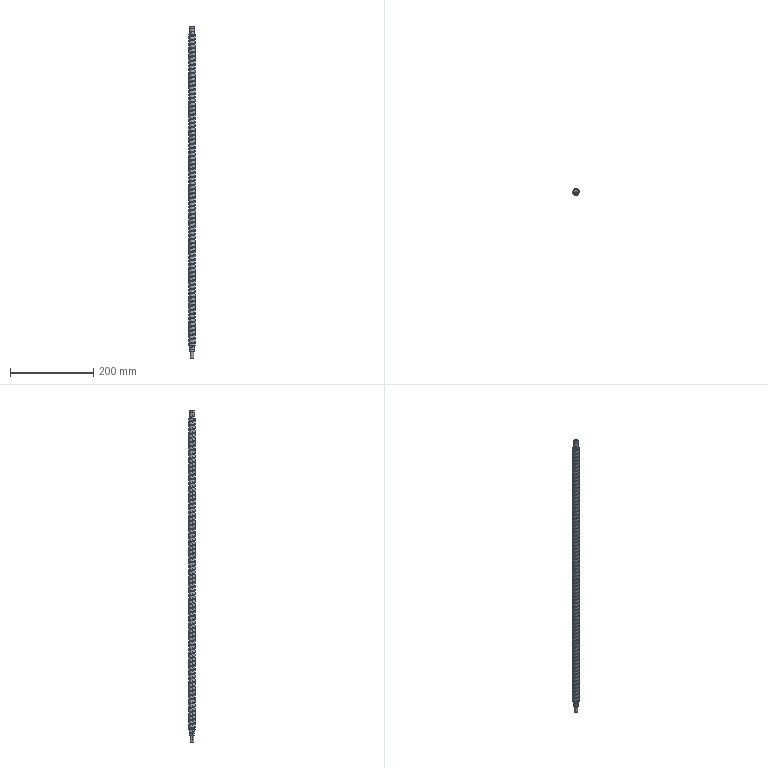Part | STEP file | 350 Lead screw | 1 solid | 182 faces | box 15 x 15 x 800 mm | volume 123903 mm3 | cylinder 171 | plane 7 | cone 2 | spline 2 | commonest cylinder face diameters 15 x152 12 x11 10 x4 3.3 x2 8 x2